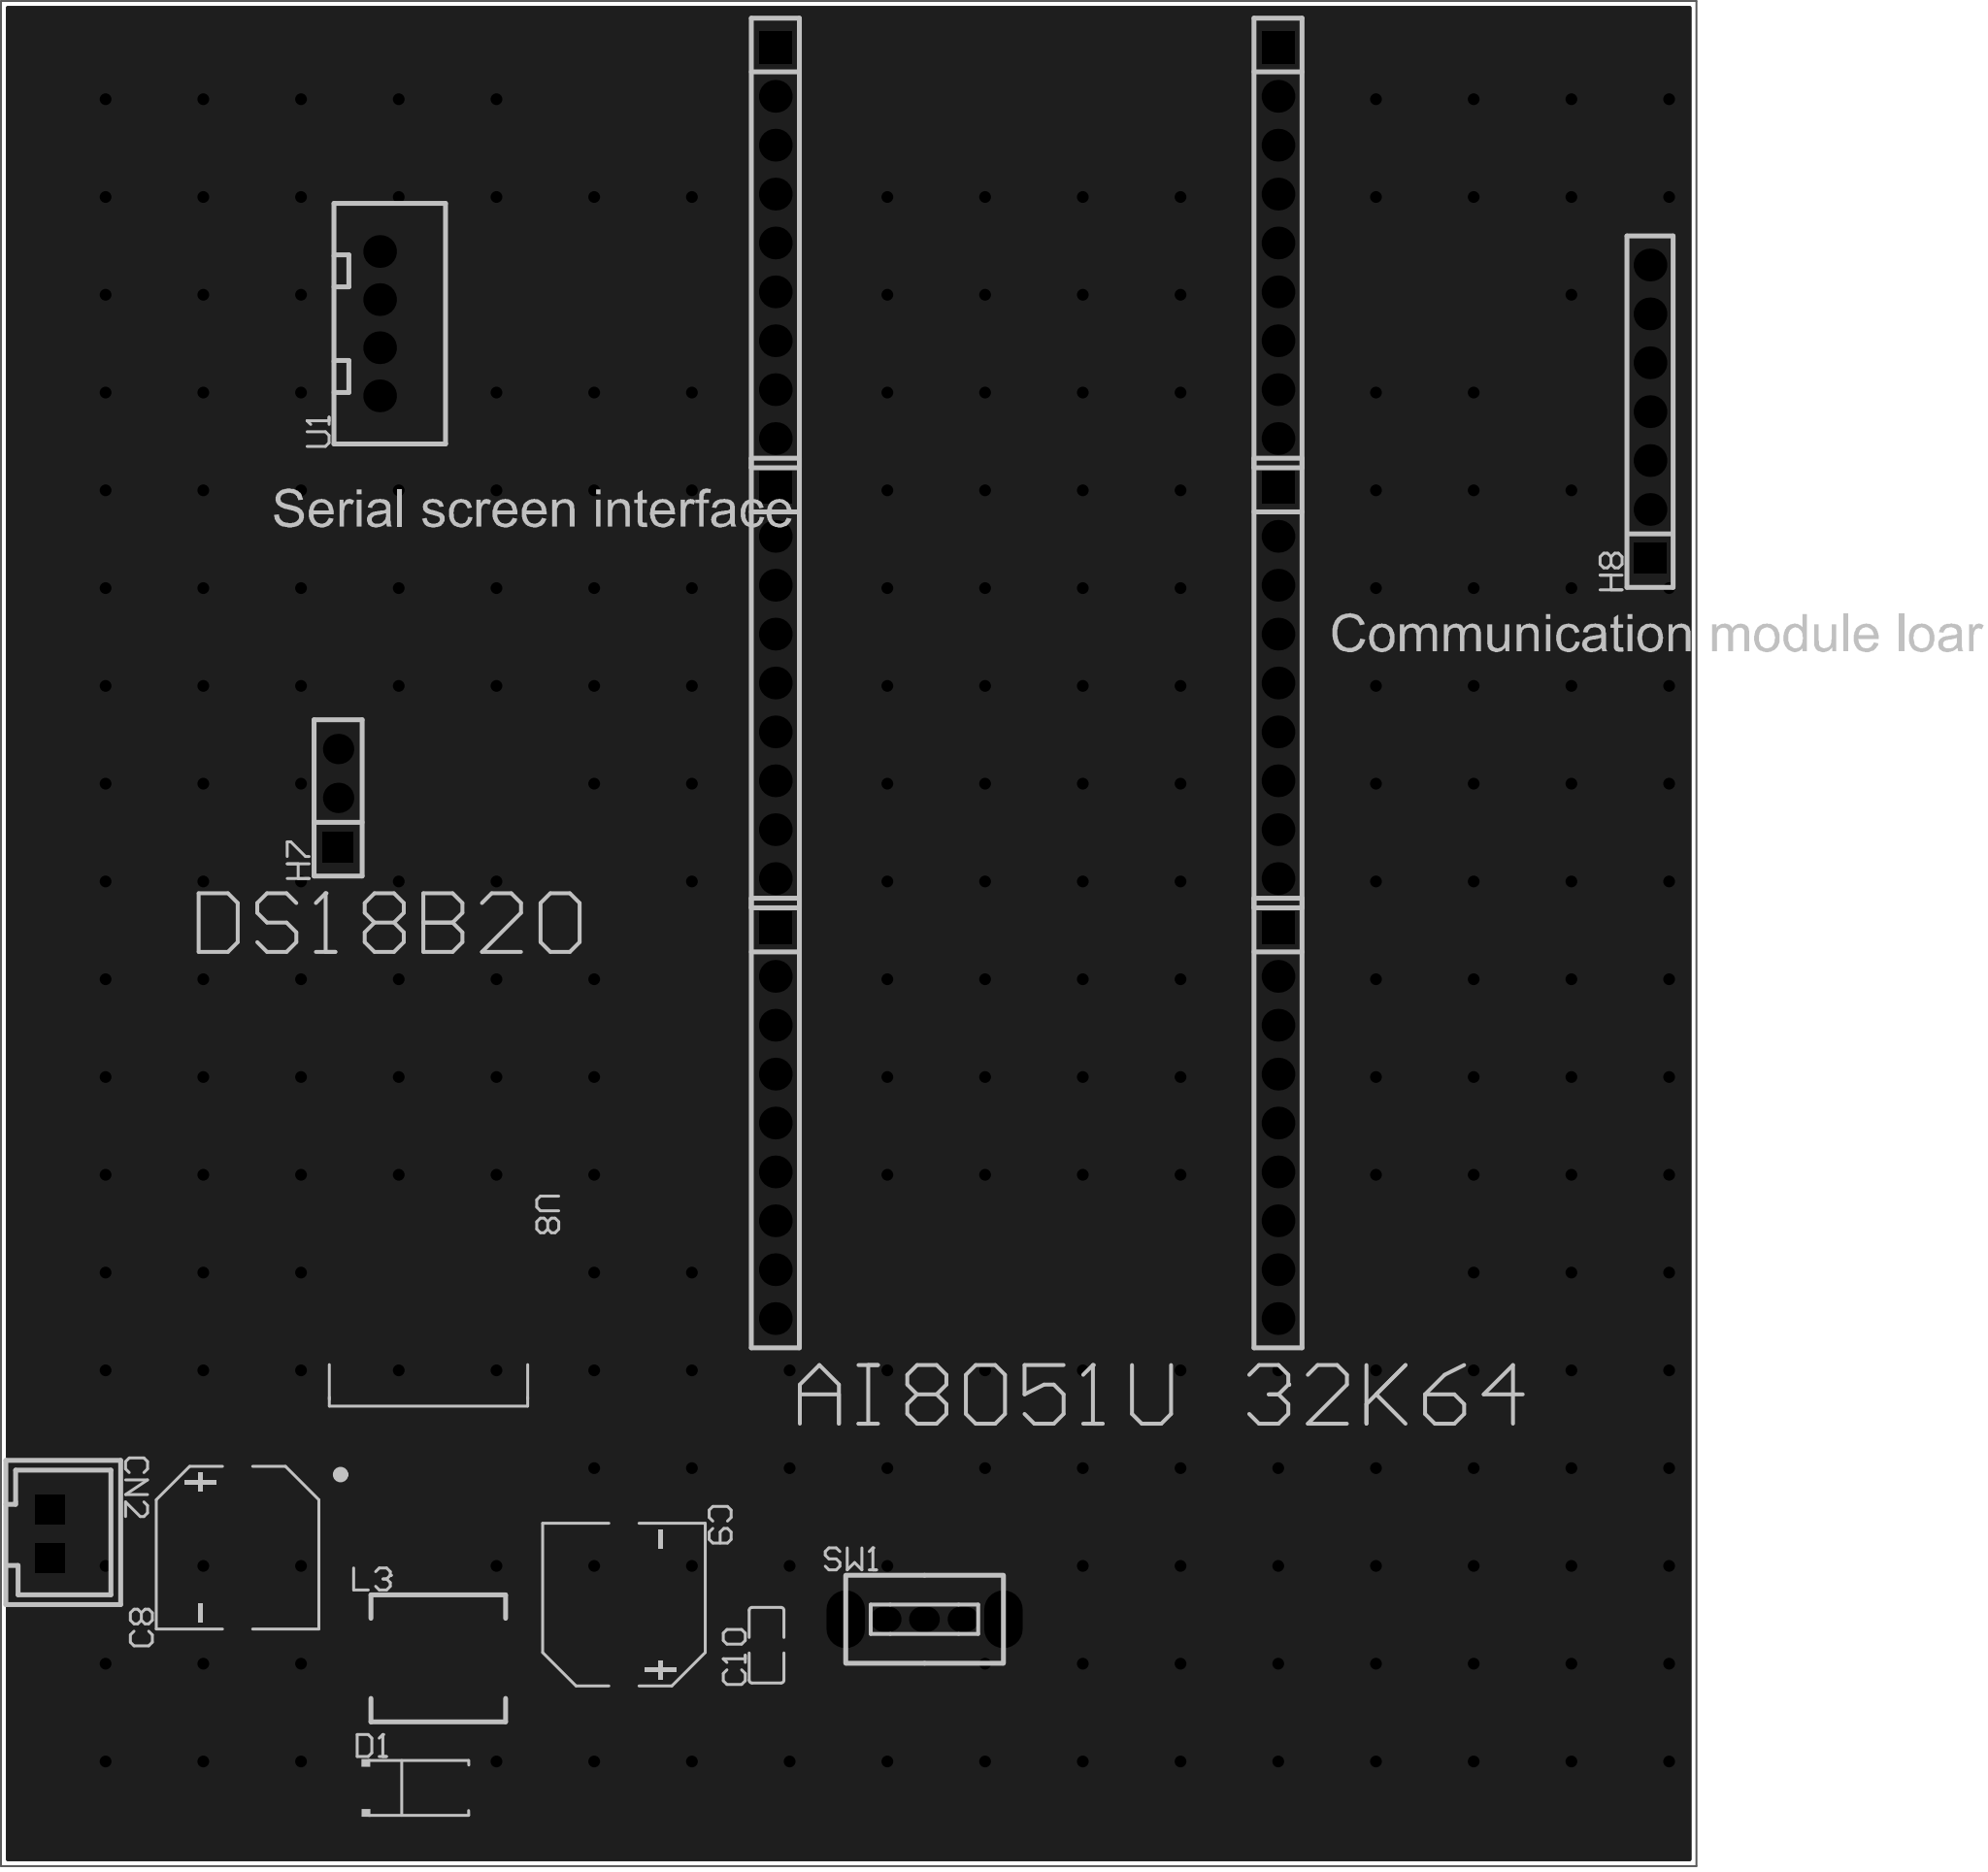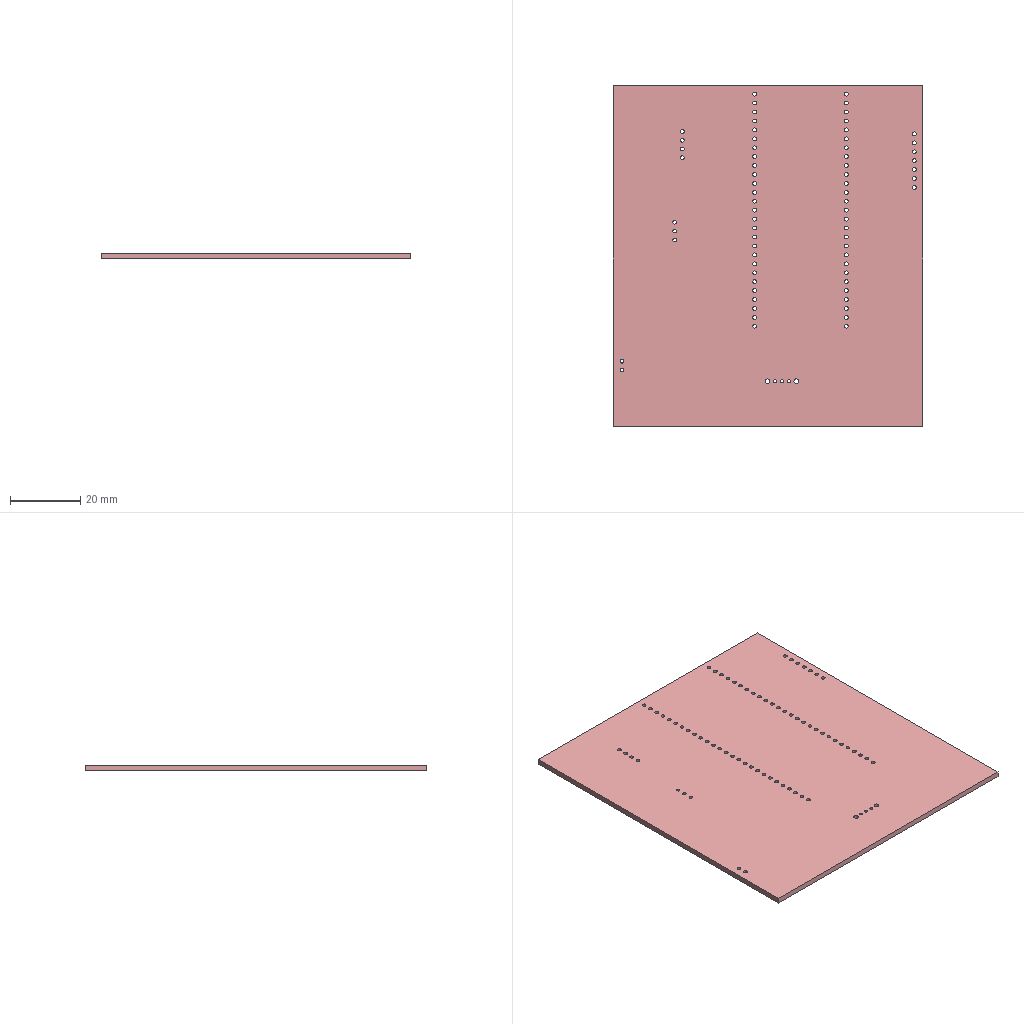Circuit board layout | Altium Designer | box 88.1 x 96.9 x 1.6 mm
Layer stack:
# Altium Designer layer stack of  (unit mm; dielectric type: 0 none, 1 core, 2 prepreg, 3 surface material)
index,name,kind,layer,copper_thickness_mm,dielectric_type,dielectric_thickness_mm,dielectric_material,dielectric_constant
0,Top Paste Mask Layer,other,,,,,,
1,Top Silkscreen Layer,other,,,,,,
2,Top Solder Mask Layer,dielectric,,,3,0.01,,3.3
3,Top Layer,copper,Top Layer,0.035,,,,
4,Dielectric1,dielectric,,,3,1.51,FR4,4.5
5,Bottom Layer,copper,Bottom Layer,0.035,,,,
6,Bottom Solder Mask Layer,dielectric,,,3,0.01,,3.3
7,Bottom Silkscreen Layer,other,,,,,,
8,Bottom Paste Mask Layer,other,,,,,,
# drill layer pairs: low layer,high layer
drill_pair,Top Layer,Bottom Layer
Part placement:
Designator,Comment,Layer,Footprint,Center-X(mm),Center-Y(mm),Rotation
C8,,TopLayer,CAP-SMD_BD8.0-L8.3-W8.3-RD,91.801,97.571,90
C9,,TopLayer,CAP-SMD_BD8.0-L8.3-W8.3-RD,111.887,94.615,270
C10,,TopLayer,C0805,119.3,92.505,90
CN2,XH2.54-2PIN-straight pin,TopLayer,CONN-TH_XH2.54-2P,82.042,98.298,270
D1,,TopLayer,SMA_L4.3-W2.6-LS5.2-RD,101.219,85.09,0
H1,,TopLayer,HDR-TH_9P-P2.54-V-F-1,119.757,165.355,270
H2,,TopLayer,HDR-TH_9P-P2.54-V-F-1,119.757,142.494,270
H3,,TopLayer,HDR-TH_9P-P2.54-V-F-1,119.757,119.634,270
H4,,TopLayer,HDR-TH_9P-P2.54-V-F-1,145.888,165.355,270
H5,,TopLayer,HDR-TH_9P-P2.54-V-F-1,145.888,142.494,270
H6,,TopLayer,HDR-TH_9P-P2.54-V-F-1,145.888,119.634,270
H7,,TopLayer,HDR-TH_3P-P2.54-V-F,97.028,136.525,90
H8,,TopLayer,HDR-TH_7P-P2.54-V-F,165.227,156.591,90
L3,,TopLayer,IND-SMD_L7.0-W6.6,102.235,91.821,0
U8,LM2596S-5.0,TopLayer,TO-263-5_L10.2-W8.9-P1.70-BR,101.727,106.426,270
U1,xh2.54-4p(straight pin),TopLayer,CONN-TH_4P-P2.50-XH2.54-4P,99.187,161.163,90
SW1,,TopLayer,拨动开关,127.516,93.853,0
Pad and via stacks:
# Altium Designer via and pad stacks of  (unit mm). Each distinct definition once, with the count of objects using it.
# via: kind,start_layer,end_layer,hole_mm,diameter_mm,mode(0 simple;1 top-mid-bottom;2 full stack),diameter_per_layer,count,example_net
# pad: kind,layer,hole_mm,hole_type(0 round;1 square;2 slot),plating,top_size,top_shape(1 round;2 rect;3 octagon;9 rounded rect),mid_size,bottom_size,mode,footprint,size_per_layer,count,example
pad,Top Layer,0,0,plated,3.61x1.26,2,3.61x1.26,3.61x1.26,0,CAP-SMD_BD8.0-L8.3-W8.3-RD,,4,C8.1
pad,Top Layer,0,0,plated,1.41x1.35,2,1.41x1.35,1.41x1.35,0,C0805,,2,C10.2
pad,Top Layer,0,0,plated,2x2,2,2x2,2x2,0,SMA_L4.3-W2.6-LS5.2-RD,,2,D1.2
pad,Top Layer,0,0,plated,2.799x3.701,2,2.799x3.701,2.799x3.701,0,IND-SMD_L7.0-W6.6,,2,L3.1
pad,Top Layer,0,0,plated,3.083x1.02,2,3.083x1.02,3.083x1.02,0,TO-263-5_L10.2-W8.9-P1.70-BR,,5,U8.1
pad,Top Layer,0,0,plated,8.5x11,2,8.5x11,8.5x11,0,TO-263-5_L10.2-W8.9-P1.70-BR,,1,U8.6
pad,Multi-Layer,1,2,plated,1.524x1.524,2,1.524x1.524,1.524x1.524,0,CONN-TH_XH2.54-2P,,2,CN2.1
pad,Multi-Layer,1.1,0,plated,1.7x1.7,2,1.7x1.7,1.7x1.7,0,HDR-TH_9P-P2.54-V-F-1,,6,H1.1
pad,Multi-Layer,1.1,0,plated,1.7x1.7,1,1.7x1.7,1.7x1.7,0,HDR-TH_9P-P2.54-V-F-1,,48,H1.2
pad,Multi-Layer,1.02,0,plated,1.575x1.575,1,1.575x1.575,1.575x1.575,0,HDR-TH_3P-P2.54-V-F,,2,H7.3
pad,Multi-Layer,1.02,0,plated,1.575x1.575,2,1.575x1.575,1.575x1.575,0,HDR-TH_3P-P2.54-V-F,,1,H7.1
pad,Multi-Layer,1.1,0,plated,1.7x1.7,1,1.7x1.7,1.7x1.7,0,HDR-TH_7P-P2.54-V-F,,6,H8.7
pad,Multi-Layer,1.1,0,plated,1.575x1.7,2,1.575x1.7,1.575x1.7,0,HDR-TH_7P-P2.54-V-F,,1,H8.1
pad,Multi-Layer,1.05,0,plated,1.7x1.7,1,1.7x1.7,1.7x1.7,0,CONN-TH_4P-P2.50-XH2.54-4P,,4,U1.1
pad,Multi-Layer,0.8992,0,plated,1.6x1.3,1,1.6x1.3,1.6x1.3,0,\u00B2\u00A6\u00B6\u00AF\u00BF\u00AA\u00B9\u00D8,,3,SW1.1
pad,Multi-Layer,1.3,0,plated,3x1.999,1,3x1.999,3x1.999,0,\u00B2\u00A6\u00B6\u00AF\u00BF\u00AA\u00B9\u00D8,,2,SW1.4
via,Top Layer,Bottom Layer,0.3048,0.61,0,,236,GND
Copper pours:
name,layer,net,type(0 solid;1 hatched;2 none)
Top Layer-GND,Top Layer,GND,0
Bottom Layer-GND,Bottom Layer,GND,0